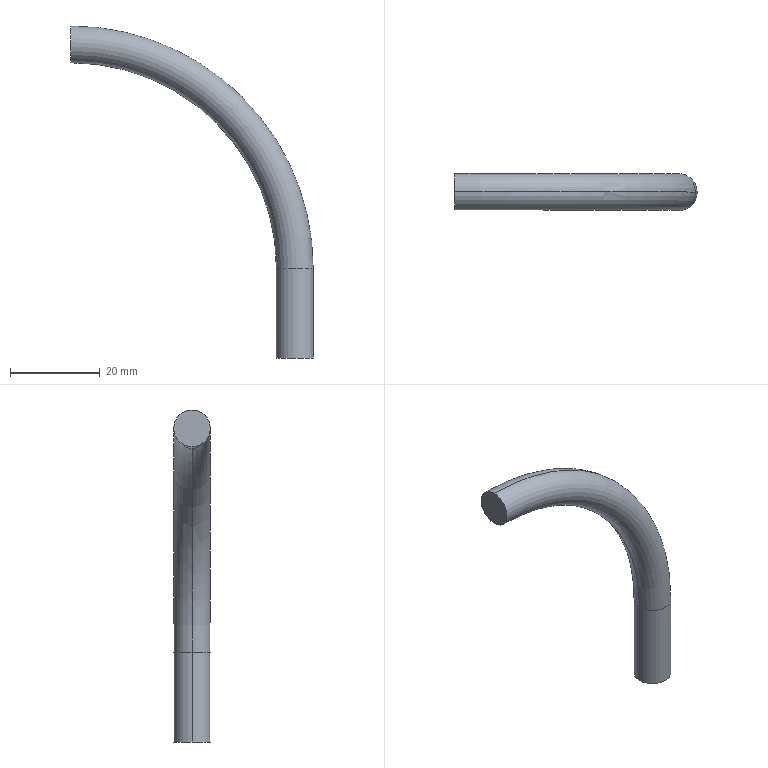Part | STEP file | ISPB-WXM-WA-750-10-650-T4-N-AQ-EB-G3-^-Part-6 | 1 solid | 6 faces | box 54.1 x 8.2 x 74.1 mm | volume 5204 mm3 | torus 2 | cylinder 2 | plane 2 | commonest cylinder face diameters 8.2 x2
STEP:
#1=CARTESIAN_POINT('',(0.,0.,0.));
#2=DIRECTION('',(0.,0.,1.));
#3=DIRECTION('',(1.,0.,0.));
#4=AXIS2_PLACEMENT_3D('',#1,#2,#3);
#5=CARTESIAN_POINT('',(351.5,14.,-8.4));
#6=VERTEX_POINT('',#5);
#7=CARTESIAN_POINT('',(351.5,14.,-0.2));
#8=VERTEX_POINT('',#7);
#9=CARTESIAN_POINT('',(351.5,14.,-4.3));
#10=DIRECTION('',(1.,0.,0.));
#11=DIRECTION('',(0.,1.,0.));
#12=AXIS2_PLACEMENT_3D('',#9,#10,#11);
#13=CIRCLE('',#12,4.1);
#14=CARTESIAN_POINT('',(351.5,14.,-54.3));
#15=DIRECTION('',(0.,1.,0.));
#16=DIRECTION('',(-1.,0.,0.));
#17=AXIS2_PLACEMENT_3D('',#14,#15,#16);
#18=TOROIDAL_SURFACE('',#17,50.,4.1);
#19=CARTESIAN_POINT('',(1.571,7.854));
#20=DIRECTION('',(0.,-1.));
#21=VECTOR('',#20,1.);
#22=LINE('',#19,#21);
#23=(GEOMETRIC_REPRESENTATION_CONTEXT(2)PARAMETRIC_REPRESENTATION_CONTEXT()REPRESENTATION_CONTEXT('',''));
#24=DEFINITIONAL_REPRESENTATION('',(#22),#23);
#25=PCURVE('',#18,#24);
#26=CARTESIAN_POINT('',(351.5,14.,-4.3));
#27=DIRECTION('',(1.,0.,0.));
#28=DIRECTION('',(0.,1.,0.));
#29=AXIS2_PLACEMENT_3D('',#26,#27,#28);
#30=PLANE('',#29);
#31=CARTESIAN_POINT('',(0.,0.));
#32=DIRECTION('',(1.,0.));
#33=AXIS2_PLACEMENT_2D('',#31,#32);
#34=CIRCLE('',#33,4.1);
#35=(GEOMETRIC_REPRESENTATION_CONTEXT(2)PARAMETRIC_REPRESENTATION_CONTEXT()REPRESENTATION_CONTEXT('',''));
#36=DEFINITIONAL_REPRESENTATION('',(#34),#35);
#37=PCURVE('',#30,#36);
#38=SURFACE_CURVE('',#13,(#25,#37),.PCURVE_S1.);
#39=EDGE_CURVE('',#6,#8,#38,.T.);
#40=ORIENTED_EDGE('',*,*,#39,.T.);
#41=CARTESIAN_POINT('',(405.6,14.,-54.3));
#42=VERTEX_POINT('',#41);
#43=CARTESIAN_POINT('',(351.5,14.,-54.3));
#44=DIRECTION('',(0.,1.,0.));
#45=DIRECTION('',(0.,0.,1.));
#46=AXIS2_PLACEMENT_3D('',#43,#44,#45);
#47=CIRCLE('',#46,54.1);
#48=CARTESIAN_POINT('',(1.571,0.));
#49=DIRECTION('',(1.,0.));
#50=VECTOR('',#49,1.);
#51=LINE('',#48,#50);
#52=(GEOMETRIC_REPRESENTATION_CONTEXT(2)PARAMETRIC_REPRESENTATION_CONTEXT()REPRESENTATION_CONTEXT('',''));
#53=DEFINITIONAL_REPRESENTATION('',(#51),#52);
#54=PCURVE('',#18,#53);
#55=CARTESIAN_POINT('',(351.5,14.,-54.3));
#56=DIRECTION('',(0.,1.,0.));
#57=DIRECTION('',(-1.,0.,0.));
#58=AXIS2_PLACEMENT_3D('',#55,#56,#57);
#59=TOROIDAL_SURFACE('',#58,50.,4.1);
#60=CARTESIAN_POINT('',(1.571,6.283));
#61=DIRECTION('',(1.,0.));
#62=VECTOR('',#61,1.);
#63=LINE('',#60,#62);
#64=(GEOMETRIC_REPRESENTATION_CONTEXT(2)PARAMETRIC_REPRESENTATION_CONTEXT()REPRESENTATION_CONTEXT('',''));
#65=DEFINITIONAL_REPRESENTATION('',(#63),#64);
#66=PCURVE('',#59,#65);
#67=SURFACE_CURVE('',#47,(#54,#66),.PCURVE_S1.);
#68=EDGE_CURVE('',#8,#42,#67,.T.);
#69=ORIENTED_EDGE('',*,*,#68,.T.);
#70=CARTESIAN_POINT('',(397.4,14.,-54.3));
#71=VERTEX_POINT('',#70);
#72=CARTESIAN_POINT('',(401.5,14.,-54.3));
#73=DIRECTION('',(0.,0.,-1.));
#74=DIRECTION('',(0.,1.,0.));
#75=AXIS2_PLACEMENT_3D('',#72,#73,#74);
#76=CIRCLE('',#75,4.1);
#77=CARTESIAN_POINT('',(3.142,7.854));
#78=DIRECTION('',(0.,-1.));
#79=VECTOR('',#78,1.);
#80=LINE('',#77,#79);
#81=(GEOMETRIC_REPRESENTATION_CONTEXT(2)PARAMETRIC_REPRESENTATION_CONTEXT()REPRESENTATION_CONTEXT('',''));
#82=DEFINITIONAL_REPRESENTATION('',(#80),#81);
#83=PCURVE('',#18,#82);
#84=CARTESIAN_POINT('',(401.5,14.,-54.3));
#85=DIRECTION('',(0.,0.,-1.));
#86=DIRECTION('',(1.,0.,0.));
#87=AXIS2_PLACEMENT_3D('',#84,#85,#86);
#88=CYLINDRICAL_SURFACE('',#87,4.1);
#89=CARTESIAN_POINT('',(-1.571,0.));
#90=DIRECTION('',(1.,0.));
#91=VECTOR('',#90,1.);
#92=LINE('',#89,#91);
#93=(GEOMETRIC_REPRESENTATION_CONTEXT(2)PARAMETRIC_REPRESENTATION_CONTEXT()REPRESENTATION_CONTEXT('',''));
#94=DEFINITIONAL_REPRESENTATION('',(#92),#93);
#95=PCURVE('',#88,#94);
#96=SURFACE_CURVE('',#76,(#83,#95),.PCURVE_S1.);
#97=EDGE_CURVE('',#71,#42,#96,.T.);
#98=ORIENTED_EDGE('',*,*,#97,.F.);
#99=CARTESIAN_POINT('',(351.5,14.,-54.3));
#100=DIRECTION('',(0.,1.,0.));
#101=DIRECTION('',(0.,0.,1.));
#102=AXIS2_PLACEMENT_3D('',#99,#100,#101);
#103=CIRCLE('',#102,45.9);
#104=CARTESIAN_POINT('',(1.571,3.142));
#105=DIRECTION('',(1.,0.));
#106=VECTOR('',#105,1.);
#107=LINE('',#104,#106);
#108=(GEOMETRIC_REPRESENTATION_CONTEXT(2)PARAMETRIC_REPRESENTATION_CONTEXT()REPRESENTATION_CONTEXT('',''));
#109=DEFINITIONAL_REPRESENTATION('',(#107),#108);
#110=PCURVE('',#18,#109);
#111=CARTESIAN_POINT('',(1.571,3.142));
#112=DIRECTION('',(1.,0.));
#113=VECTOR('',#112,1.);
#114=LINE('',#111,#113);
#115=(GEOMETRIC_REPRESENTATION_CONTEXT(2)PARAMETRIC_REPRESENTATION_CONTEXT()REPRESENTATION_CONTEXT('',''));
#116=DEFINITIONAL_REPRESENTATION('',(#114),#115);
#117=PCURVE('',#59,#116);
#118=SURFACE_CURVE('',#103,(#110,#117),.PCURVE_S1.);
#119=EDGE_CURVE('',#6,#71,#118,.T.);
#120=ORIENTED_EDGE('',*,*,#119,.F.);
#121=EDGE_LOOP('',(#40,#69,#98,#120));
#122=FACE_BOUND('',#121,.T.);
#123=ADVANCED_FACE('',(#122),#18,.T.);
#124=CARTESIAN_POINT('',(401.5,14.,-54.3));
#125=DIRECTION('',(0.,0.,-1.));
#126=DIRECTION('',(0.,1.,0.));
#127=AXIS2_PLACEMENT_3D('',#124,#125,#126);
#128=CIRCLE('',#127,4.1);
#129=CARTESIAN_POINT('',(401.5,14.,-54.3));
#130=DIRECTION('',(0.,0.,-1.));
#131=DIRECTION('',(1.,0.,0.));
#132=AXIS2_PLACEMENT_3D('',#129,#130,#131);
#133=CYLINDRICAL_SURFACE('',#132,4.1);
#134=CARTESIAN_POINT('',(-1.571,0.));
#135=DIRECTION('',(1.,0.));
#136=VECTOR('',#135,1.);
#137=LINE('',#134,#136);
#138=(GEOMETRIC_REPRESENTATION_CONTEXT(2)PARAMETRIC_REPRESENTATION_CONTEXT()REPRESENTATION_CONTEXT('',''));
#139=DEFINITIONAL_REPRESENTATION('',(#137),#138);
#140=PCURVE('',#133,#139);
#141=CARTESIAN_POINT('',(3.142,7.854));
#142=DIRECTION('',(0.,-1.));
#143=VECTOR('',#142,1.);
#144=LINE('',#141,#143);
#145=(GEOMETRIC_REPRESENTATION_CONTEXT(2)PARAMETRIC_REPRESENTATION_CONTEXT()REPRESENTATION_CONTEXT('',''));
#146=DEFINITIONAL_REPRESENTATION('',(#144),#145);
#147=PCURVE('',#59,#146);
#148=SURFACE_CURVE('',#128,(#140,#147),.PCURVE_S1.);
#149=EDGE_CURVE('',#42,#71,#148,.T.);
#150=ORIENTED_EDGE('',*,*,#149,.T.);
#151=CARTESIAN_POINT('',(397.4,14.,-74.3));
#152=VERTEX_POINT('',#151);
#153=CARTESIAN_POINT('',(397.4,14.,-54.3));
#154=DIRECTION('',(0.,0.,-1.));
#155=VECTOR('',#154,1.);
#156=LINE('',#153,#155);
#157=CARTESIAN_POINT('',(3.142,0.));
#158=DIRECTION('',(0.,1.));
#159=VECTOR('',#158,1.);
#160=LINE('',#157,#159);
#161=(GEOMETRIC_REPRESENTATION_CONTEXT(2)PARAMETRIC_REPRESENTATION_CONTEXT()REPRESENTATION_CONTEXT('',''));
#162=DEFINITIONAL_REPRESENTATION('',(#160),#161);
#163=PCURVE('',#133,#162);
#164=CARTESIAN_POINT('',(3.142,0.));
#165=DIRECTION('',(0.,1.));
#166=VECTOR('',#165,1.);
#167=LINE('',#164,#166);
#168=(GEOMETRIC_REPRESENTATION_CONTEXT(2)PARAMETRIC_REPRESENTATION_CONTEXT()REPRESENTATION_CONTEXT('',''));
#169=DEFINITIONAL_REPRESENTATION('',(#167),#168);
#170=PCURVE('',#88,#169);
#171=SURFACE_CURVE('',#156,(#163,#170),.PCURVE_S1.);
#172=EDGE_CURVE('',#71,#152,#171,.T.);
#173=ORIENTED_EDGE('',*,*,#172,.T.);
#174=CARTESIAN_POINT('',(405.6,14.,-74.3));
#175=VERTEX_POINT('',#174);
#176=CARTESIAN_POINT('',(401.5,14.,-74.3));
#177=DIRECTION('',(0.,0.,1.));
#178=DIRECTION('',(-1.,0.,0.));
#179=AXIS2_PLACEMENT_3D('',#176,#177,#178);
#180=CIRCLE('',#179,4.1);
#181=CARTESIAN_POINT('',(3.142,20.));
#182=DIRECTION('',(-1.,0.));
#183=VECTOR('',#182,1.);
#184=LINE('',#181,#183);
#185=(GEOMETRIC_REPRESENTATION_CONTEXT(2)PARAMETRIC_REPRESENTATION_CONTEXT()REPRESENTATION_CONTEXT('',''));
#186=DEFINITIONAL_REPRESENTATION('',(#184),#185);
#187=PCURVE('',#133,#186);
#188=CARTESIAN_POINT('',(401.5,14.,-74.3));
#189=DIRECTION('',(0.,0.,-1.));
#190=DIRECTION('',(1.,0.,0.));
#191=AXIS2_PLACEMENT_3D('',#188,#189,#190);
#192=PLANE('',#191);
#193=CARTESIAN_POINT('',(-4.1,0.));
#194=CARTESIAN_POINT('',(-4.1,7.101));
#195=CARTESIAN_POINT('',(2.05,3.551));
#196=CARTESIAN_POINT('',(8.2,0.));
#197=CARTESIAN_POINT('',(2.05,-3.551));
#198=CARTESIAN_POINT('',(-4.1,-7.101));
#199=CARTESIAN_POINT('',(-4.1,0.));
#200=(BOUNDED_CURVE()B_SPLINE_CURVE(2,(#193,#194,#195,#196,#197,#198,#199),.UNSPECIFIED.,.T.,.F.)B_SPLINE_CURVE_WITH_KNOTS((1,2,2,2,2,1),(-2.094,0.,2.094,4.189,6.283,8.378),.UNSPECIFIED.)CURVE()GEOMETRIC_REPRESENTATION_ITEM()RATIONAL_B_SPLINE_CURVE((1.,0.5,1.,0.5,1.,0.5,1.))REPRESENTATION_ITEM(''));
#201=(GEOMETRIC_REPRESENTATION_CONTEXT(2)PARAMETRIC_REPRESENTATION_CONTEXT()REPRESENTATION_CONTEXT('',''));
#202=DEFINITIONAL_REPRESENTATION('',(#200),#201);
#203=PCURVE('',#192,#202);
#204=SURFACE_CURVE('',#180,(#187,#203),.PCURVE_S1.);
#205=EDGE_CURVE('',#152,#175,#204,.T.);
#206=ORIENTED_EDGE('',*,*,#205,.T.);
#207=CARTESIAN_POINT('',(405.6,14.,-54.3));
#208=DIRECTION('',(0.,0.,-1.));
#209=VECTOR('',#208,1.);
#210=LINE('',#207,#209);
#211=CARTESIAN_POINT('',(0.,0.));
#212=DIRECTION('',(0.,1.));
#213=VECTOR('',#212,1.);
#214=LINE('',#211,#213);
#215=(GEOMETRIC_REPRESENTATION_CONTEXT(2)PARAMETRIC_REPRESENTATION_CONTEXT()REPRESENTATION_CONTEXT('',''));
#216=DEFINITIONAL_REPRESENTATION('',(#214),#215);
#217=PCURVE('',#133,#216);
#218=CARTESIAN_POINT('',(6.283,0.));
#219=DIRECTION('',(0.,1.));
#220=VECTOR('',#219,1.);
#221=LINE('',#218,#220);
#222=(GEOMETRIC_REPRESENTATION_CONTEXT(2)PARAMETRIC_REPRESENTATION_CONTEXT()REPRESENTATION_CONTEXT('',''));
#223=DEFINITIONAL_REPRESENTATION('',(#221),#222);
#224=PCURVE('',#88,#223);
#225=SURFACE_CURVE('',#210,(#217,#224),.PCURVE_S1.);
#226=EDGE_CURVE('',#42,#175,#225,.T.);
#227=ORIENTED_EDGE('',*,*,#226,.F.);
#228=EDGE_LOOP('',(#150,#173,#206,#227));
#229=FACE_BOUND('',#228,.T.);
#230=ADVANCED_FACE('',(#229),#133,.T.);
#231=ORIENTED_EDGE('',*,*,#68,.F.);
#232=CARTESIAN_POINT('',(351.5,14.,-4.3));
#233=DIRECTION('',(1.,0.,0.));
#234=DIRECTION('',(0.,1.,0.));
#235=AXIS2_PLACEMENT_3D('',#232,#233,#234);
#236=CIRCLE('',#235,4.1);
#237=CARTESIAN_POINT('',(1.571,7.854));
#238=DIRECTION('',(0.,-1.));
#239=VECTOR('',#238,1.);
#240=LINE('',#237,#239);
#241=(GEOMETRIC_REPRESENTATION_CONTEXT(2)PARAMETRIC_REPRESENTATION_CONTEXT()REPRESENTATION_CONTEXT('',''));
#242=DEFINITIONAL_REPRESENTATION('',(#240),#241);
#243=PCURVE('',#59,#242);
#244=CARTESIAN_POINT('',(0.,0.));
#245=DIRECTION('',(1.,0.));
#246=AXIS2_PLACEMENT_2D('',#244,#245);
#247=CIRCLE('',#246,4.1);
#248=(GEOMETRIC_REPRESENTATION_CONTEXT(2)PARAMETRIC_REPRESENTATION_CONTEXT()REPRESENTATION_CONTEXT('',''));
#249=DEFINITIONAL_REPRESENTATION('',(#247),#248);
#250=PCURVE('',#30,#249);
#251=SURFACE_CURVE('',#236,(#243,#250),.PCURVE_S1.);
#252=EDGE_CURVE('',#8,#6,#251,.T.);
#253=ORIENTED_EDGE('',*,*,#252,.T.);
#254=ORIENTED_EDGE('',*,*,#119,.T.);
#255=ORIENTED_EDGE('',*,*,#149,.F.);
#256=EDGE_LOOP('',(#231,#253,#254,#255));
#257=FACE_BOUND('',#256,.T.);
#258=ADVANCED_FACE('',(#257),#59,.T.);
#259=ORIENTED_EDGE('',*,*,#39,.F.);
#260=ORIENTED_EDGE('',*,*,#252,.F.);
#261=EDGE_LOOP('',(#259,#260));
#262=FACE_BOUND('',#261,.T.);
#263=ADVANCED_FACE('',(#262),#30,.F.);
#264=CARTESIAN_POINT('',(401.5,14.,-74.3));
#265=DIRECTION('',(0.,0.,1.));
#266=DIRECTION('',(-1.,0.,0.));
#267=AXIS2_PLACEMENT_3D('',#264,#265,#266);
#268=CIRCLE('',#267,4.1);
#269=CARTESIAN_POINT('',(-4.1,0.));
#270=CARTESIAN_POINT('',(-4.1,7.101));
#271=CARTESIAN_POINT('',(2.05,3.551));
#272=CARTESIAN_POINT('',(8.2,0.));
#273=CARTESIAN_POINT('',(2.05,-3.551));
#274=CARTESIAN_POINT('',(-4.1,-7.101));
#275=CARTESIAN_POINT('',(-4.1,0.));
#276=(BOUNDED_CURVE()B_SPLINE_CURVE(2,(#269,#270,#271,#272,#273,#274,#275),.UNSPECIFIED.,.T.,.F.)B_SPLINE_CURVE_WITH_KNOTS((1,2,2,2,2,1),(-2.094,0.,2.094,4.189,6.283,8.378),.UNSPECIFIED.)CURVE()GEOMETRIC_REPRESENTATION_ITEM()RATIONAL_B_SPLINE_CURVE((1.,0.5,1.,0.5,1.,0.5,1.))REPRESENTATION_ITEM(''));
#277=(GEOMETRIC_REPRESENTATION_CONTEXT(2)PARAMETRIC_REPRESENTATION_CONTEXT()REPRESENTATION_CONTEXT('',''));
#278=DEFINITIONAL_REPRESENTATION('',(#276),#277);
#279=PCURVE('',#192,#278);
#280=CARTESIAN_POINT('',(9.425,20.));
#281=DIRECTION('',(-1.,0.));
#282=VECTOR('',#281,1.);
#283=LINE('',#280,#282);
#284=(GEOMETRIC_REPRESENTATION_CONTEXT(2)PARAMETRIC_REPRESENTATION_CONTEXT()REPRESENTATION_CONTEXT('',''));
#285=DEFINITIONAL_REPRESENTATION('',(#283),#284);
#286=PCURVE('',#88,#285);
#287=SURFACE_CURVE('',#268,(#279,#286),.PCURVE_S1.);
#288=EDGE_CURVE('',#175,#152,#287,.T.);
#289=ORIENTED_EDGE('',*,*,#288,.F.);
#290=ORIENTED_EDGE('',*,*,#205,.F.);
#291=EDGE_LOOP('',(#289,#290));
#292=FACE_BOUND('',#291,.T.);
#293=ADVANCED_FACE('',(#292),#192,.T.);
#294=ORIENTED_EDGE('',*,*,#172,.F.);
#295=ORIENTED_EDGE('',*,*,#97,.T.);
#296=ORIENTED_EDGE('',*,*,#226,.T.);
#297=ORIENTED_EDGE('',*,*,#288,.T.);
#298=EDGE_LOOP('',(#294,#295,#296,#297));
#299=FACE_BOUND('',#298,.T.);
#300=ADVANCED_FACE('',(#299),#88,.T.);
#301=CLOSED_SHELL('',(#123,#230,#258,#263,#293,#300));
#302=MANIFOLD_SOLID_BREP('',#301);
#303=(LENGTH_UNIT()NAMED_UNIT(*)SI_UNIT(.MILLI.,.METRE.));
#304=UNCERTAINTY_MEASURE_WITH_UNIT(LENGTH_MEASURE(0.0000001),#303,'','');
#305=(NAMED_UNIT(*)PLANE_ANGLE_UNIT()SI_UNIT($,.RADIAN.));
#306=(NAMED_UNIT(*)SI_UNIT($,.STERADIAN.)SOLID_ANGLE_UNIT());
#307=(GEOMETRIC_REPRESENTATION_CONTEXT(3)GLOBAL_UNCERTAINTY_ASSIGNED_CONTEXT((#304))GLOBAL_UNIT_ASSIGNED_CONTEXT((#303,#305,#306))REPRESENTATION_CONTEXT('',''));
#308=ADVANCED_BREP_SHAPE_REPRESENTATION('',(#4,#302),#307);